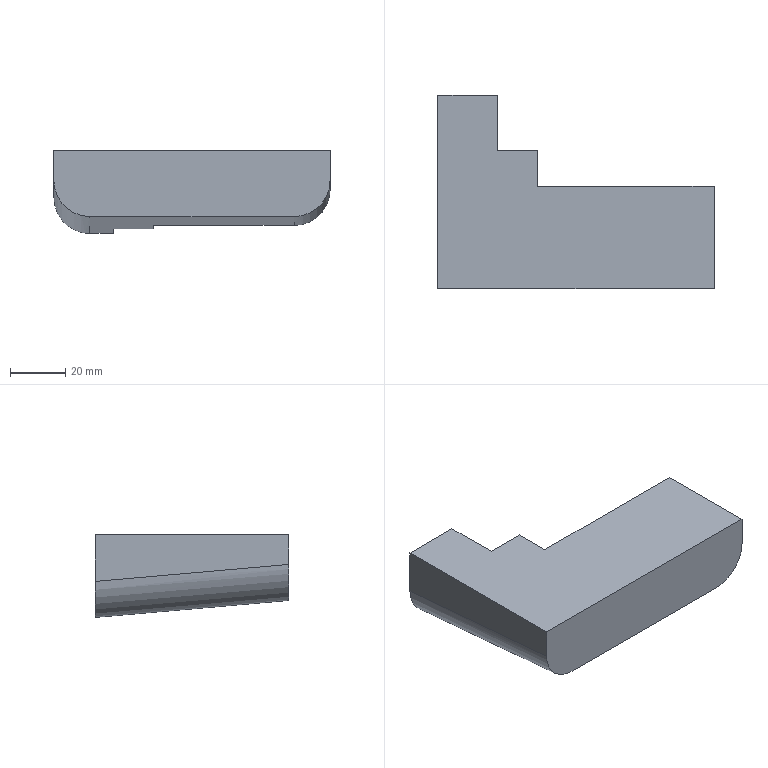Part | STEP file | 1 solid | 12 faces | box 100 x 70 x 30 mm | volume 115912 mm3 | plane 10 | cylinder 2 | commonest cylinder face diameters 26 x2
STEP:
#1=CARTESIAN_POINT('',(0.,0.,0.));
#2=DIRECTION('',(0.,0.,1.));
#3=DIRECTION('',(1.,0.,0.));
#4=AXIS2_PLACEMENT_3D('',#1,#2,#3);
#5=CARTESIAN_POINT('',(-86.362,50.,-64.721));
#6=VERTEX_POINT('',#5);
#7=CARTESIAN_POINT('',(-86.362,37.,-63.583));
#8=VERTEX_POINT('',#7);
#9=CARTESIAN_POINT('',(-86.362,70.,-66.47));
#10=DIRECTION('',(0.,-0.9962,0.08716));
#11=VECTOR('',#10,1.);
#12=LINE('',#9,#11);
#13=CARTESIAN_POINT('',(-72.362,70.,-66.47));
#14=DIRECTION('',(0.,0.08716,0.9962));
#15=DIRECTION('',(0.,-0.9962,0.08716));
#16=AXIS2_PLACEMENT_3D('',#13,#14,#15);
#17=PLANE('',#16);
#18=CARTESIAN_POINT('',(0.,-14.));
#19=DIRECTION('',(1.,0.));
#20=VECTOR('',#19,1.);
#21=LINE('',#18,#20);
#22=(GEOMETRIC_REPRESENTATION_CONTEXT(2)PARAMETRIC_REPRESENTATION_CONTEXT()REPRESENTATION_CONTEXT('',''));
#23=DEFINITIONAL_REPRESENTATION('',(#21),#22);
#24=PCURVE('',#17,#23);
#25=CARTESIAN_POINT('',(-86.362,0.,-92.47));
#26=DIRECTION('',(-1.,0.,0.));
#27=DIRECTION('',(0.,0.,1.));
#28=AXIS2_PLACEMENT_3D('',#25,#26,#27);
#29=PLANE('',#28);
#30=CARTESIAN_POINT('',(26.,70.));
#31=DIRECTION('',(0.08716,-0.9962));
#32=VECTOR('',#31,1.);
#33=LINE('',#30,#32);
#34=(GEOMETRIC_REPRESENTATION_CONTEXT(2)PARAMETRIC_REPRESENTATION_CONTEXT()REPRESENTATION_CONTEXT('',''));
#35=DEFINITIONAL_REPRESENTATION('',(#33),#34);
#36=PCURVE('',#29,#35);
#37=SURFACE_CURVE('',#12,(#24,#36),.PCURVE_S1.);
#38=EDGE_CURVE('',#6,#8,#37,.T.);
#39=ORIENTED_EDGE('',*,*,#38,.T.);
#40=CARTESIAN_POINT('',(-35.362,37.,-63.583));
#41=VERTEX_POINT('',#40);
#42=CARTESIAN_POINT('',(-72.362,37.,-63.583));
#43=DIRECTION('',(-1.,0.,0.));
#44=VECTOR('',#43,1.);
#45=LINE('',#42,#44);
#46=CARTESIAN_POINT('',(33.126,0.));
#47=DIRECTION('',(0.,-1.));
#48=VECTOR('',#47,1.);
#49=LINE('',#46,#48);
#50=(GEOMETRIC_REPRESENTATION_CONTEXT(2)PARAMETRIC_REPRESENTATION_CONTEXT()REPRESENTATION_CONTEXT('',''));
#51=DEFINITIONAL_REPRESENTATION('',(#49),#50);
#52=PCURVE('',#17,#51);
#53=CARTESIAN_POINT('',(-42.862,37.,-64.47));
#54=DIRECTION('',(0.,1.,0.));
#55=DIRECTION('',(0.,0.,1.));
#56=AXIS2_PLACEMENT_3D('',#53,#54,#55);
#57=PLANE('',#56);
#58=CARTESIAN_POINT('',(0.8871,-29.5));
#59=DIRECTION('',(0.,-1.));
#60=VECTOR('',#59,1.);
#61=LINE('',#58,#60);
#62=(GEOMETRIC_REPRESENTATION_CONTEXT(2)PARAMETRIC_REPRESENTATION_CONTEXT()REPRESENTATION_CONTEXT('',''));
#63=DEFINITIONAL_REPRESENTATION('',(#61),#62);
#64=PCURVE('',#57,#63);
#65=SURFACE_CURVE('',#45,(#52,#64),.PCURVE_S1.);
#66=EDGE_CURVE('',#41,#8,#65,.T.);
#67=ORIENTED_EDGE('',*,*,#66,.F.);
#68=CARTESIAN_POINT('',(-35.362,0.,-60.346));
#69=VERTEX_POINT('',#68);
#70=CARTESIAN_POINT('',(-35.362,70.,-66.47));
#71=DIRECTION('',(0.,0.9962,-0.08716));
#72=VECTOR('',#71,1.);
#73=LINE('',#70,#72);
#74=CARTESIAN_POINT('',(0.,37.));
#75=DIRECTION('',(-1.,0.));
#76=VECTOR('',#75,1.);
#77=LINE('',#74,#76);
#78=(GEOMETRIC_REPRESENTATION_CONTEXT(2)PARAMETRIC_REPRESENTATION_CONTEXT()REPRESENTATION_CONTEXT('',''));
#79=DEFINITIONAL_REPRESENTATION('',(#77),#78);
#80=PCURVE('',#17,#79);
#81=CARTESIAN_POINT('',(-35.362,149.657,-60.39));
#82=DIRECTION('',(0.,-0.9962,0.08716));
#83=DIRECTION('',(0.,-0.08716,-0.9962));
#84=AXIS2_PLACEMENT_3D('',#81,#82,#83);
#85=CYLINDRICAL_SURFACE('',#84,13.);
#86=CARTESIAN_POINT('',(0.,78.824));
#87=DIRECTION('',(0.,-1.));
#88=VECTOR('',#87,1.);
#89=LINE('',#86,#88);
#90=(GEOMETRIC_REPRESENTATION_CONTEXT(2)PARAMETRIC_REPRESENTATION_CONTEXT()REPRESENTATION_CONTEXT('',''));
#91=DEFINITIONAL_REPRESENTATION('',(#89),#90);
#92=PCURVE('',#85,#91);
#93=SURFACE_CURVE('',#73,(#80,#92),.PCURVE_S1.);
#94=EDGE_CURVE('',#69,#41,#93,.T.);
#95=ORIENTED_EDGE('',*,*,#94,.F.);
#96=CARTESIAN_POINT('',(-109.362,0.,-60.346));
#97=VERTEX_POINT('',#96);
#98=CARTESIAN_POINT('',(-72.362,0.,-60.346));
#99=DIRECTION('',(1.,0.,0.));
#100=VECTOR('',#99,1.);
#101=LINE('',#98,#100);
#102=CARTESIAN_POINT('',(70.267,0.));
#103=DIRECTION('',(0.,1.));
#104=VECTOR('',#103,1.);
#105=LINE('',#102,#104);
#106=(GEOMETRIC_REPRESENTATION_CONTEXT(2)PARAMETRIC_REPRESENTATION_CONTEXT()REPRESENTATION_CONTEXT('',''));
#107=DEFINITIONAL_REPRESENTATION('',(#105),#106);
#108=PCURVE('',#17,#107);
#109=CARTESIAN_POINT('',(-72.362,0.,-51.47));
#110=DIRECTION('',(0.,1.,0.));
#111=DIRECTION('',(-1.,0.,0.));
#112=AXIS2_PLACEMENT_3D('',#109,#110,#111);
#113=PLANE('',#112);
#114=CARTESIAN_POINT('',(0.,-8.876));
#115=DIRECTION('',(-1.,0.));
#116=VECTOR('',#115,1.);
#117=LINE('',#114,#116);
#118=(GEOMETRIC_REPRESENTATION_CONTEXT(2)PARAMETRIC_REPRESENTATION_CONTEXT()REPRESENTATION_CONTEXT('',''));
#119=DEFINITIONAL_REPRESENTATION('',(#117),#118);
#120=PCURVE('',#113,#119);
#121=SURFACE_CURVE('',#101,(#108,#120),.PCURVE_S1.);
#122=EDGE_CURVE('',#97,#69,#121,.T.);
#123=ORIENTED_EDGE('',*,*,#122,.F.);
#124=CARTESIAN_POINT('',(-109.362,70.,-66.47));
#125=VERTEX_POINT('',#124);
#126=CARTESIAN_POINT('',(-109.362,70.,-66.47));
#127=DIRECTION('',(0.,-0.9962,0.08716));
#128=VECTOR('',#127,1.);
#129=LINE('',#126,#128);
#130=CARTESIAN_POINT('',(0.,-37.));
#131=DIRECTION('',(1.,0.));
#132=VECTOR('',#131,1.);
#133=LINE('',#130,#132);
#134=(GEOMETRIC_REPRESENTATION_CONTEXT(2)PARAMETRIC_REPRESENTATION_CONTEXT()REPRESENTATION_CONTEXT('',''));
#135=DEFINITIONAL_REPRESENTATION('',(#133),#134);
#136=PCURVE('',#17,#135);
#137=CARTESIAN_POINT('',(-109.362,71.133,-53.52));
#138=DIRECTION('',(0.,-0.9962,0.08716));
#139=DIRECTION('',(0.,-0.08716,-0.9962));
#140=AXIS2_PLACEMENT_3D('',#137,#138,#139);
#141=CYLINDRICAL_SURFACE('',#140,13.);
#142=CARTESIAN_POINT('',(6.283,0.));
#143=DIRECTION('',(0.,1.));
#144=VECTOR('',#143,1.);
#145=LINE('',#142,#144);
#146=(GEOMETRIC_REPRESENTATION_CONTEXT(2)PARAMETRIC_REPRESENTATION_CONTEXT()REPRESENTATION_CONTEXT('',''));
#147=DEFINITIONAL_REPRESENTATION('',(#145),#146);
#148=PCURVE('',#141,#147);
#149=SURFACE_CURVE('',#129,(#136,#148),.PCURVE_S1.);
#150=EDGE_CURVE('',#125,#97,#149,.T.);
#151=ORIENTED_EDGE('',*,*,#150,.F.);
#152=CARTESIAN_POINT('',(-100.862,70.,-66.47));
#153=VERTEX_POINT('',#152);
#154=CARTESIAN_POINT('',(-72.362,70.,-66.47));
#155=DIRECTION('',(1.,0.,0.));
#156=VECTOR('',#155,1.);
#157=LINE('',#154,#156);
#158=CARTESIAN_POINT('',(0.,0.));
#159=DIRECTION('',(0.,1.));
#160=VECTOR('',#159,1.);
#161=LINE('',#158,#160);
#162=(GEOMETRIC_REPRESENTATION_CONTEXT(2)PARAMETRIC_REPRESENTATION_CONTEXT()REPRESENTATION_CONTEXT('',''));
#163=DEFINITIONAL_REPRESENTATION('',(#161),#162);
#164=PCURVE('',#17,#163);
#165=CARTESIAN_POINT('',(469.637,70.,73.53));
#166=DIRECTION('',(0.,-1.,0.));
#167=DIRECTION('',(1.,0.,0.));
#168=AXIS2_PLACEMENT_3D('',#165,#166,#167);
#169=PLANE('',#168);
#170=CARTESIAN_POINT('',(-542.,-140.));
#171=DIRECTION('',(1.,0.));
#172=VECTOR('',#171,1.);
#173=LINE('',#170,#172);
#174=(GEOMETRIC_REPRESENTATION_CONTEXT(2)PARAMETRIC_REPRESENTATION_CONTEXT()REPRESENTATION_CONTEXT('',''));
#175=DEFINITIONAL_REPRESENTATION('',(#173),#174);
#176=PCURVE('',#169,#175);
#177=SURFACE_CURVE('',#157,(#164,#176),.PCURVE_S1.);
#178=EDGE_CURVE('',#125,#153,#177,.T.);
#179=ORIENTED_EDGE('',*,*,#178,.T.);
#180=CARTESIAN_POINT('',(-100.862,50.,-64.721));
#181=VERTEX_POINT('',#180);
#182=CARTESIAN_POINT('',(-100.862,70.,-66.47));
#183=DIRECTION('',(0.,-0.9962,0.08716));
#184=VECTOR('',#183,1.);
#185=LINE('',#182,#184);
#186=CARTESIAN_POINT('',(0.,-28.5));
#187=DIRECTION('',(1.,0.));
#188=VECTOR('',#187,1.);
#189=LINE('',#186,#188);
#190=(GEOMETRIC_REPRESENTATION_CONTEXT(2)PARAMETRIC_REPRESENTATION_CONTEXT()REPRESENTATION_CONTEXT('',''));
#191=DEFINITIONAL_REPRESENTATION('',(#189),#190);
#192=PCURVE('',#17,#191);
#193=CARTESIAN_POINT('',(-100.862,0.,-92.47));
#194=DIRECTION('',(-1.,0.,0.));
#195=DIRECTION('',(0.,0.,1.));
#196=AXIS2_PLACEMENT_3D('',#193,#194,#195);
#197=PLANE('',#196);
#198=CARTESIAN_POINT('',(26.,70.));
#199=DIRECTION('',(0.08716,-0.9962));
#200=VECTOR('',#199,1.);
#201=LINE('',#198,#200);
#202=(GEOMETRIC_REPRESENTATION_CONTEXT(2)PARAMETRIC_REPRESENTATION_CONTEXT()REPRESENTATION_CONTEXT('',''));
#203=DEFINITIONAL_REPRESENTATION('',(#201),#202);
#204=PCURVE('',#197,#203);
#205=SURFACE_CURVE('',#185,(#192,#204),.PCURVE_S1.);
#206=EDGE_CURVE('',#153,#181,#205,.T.);
#207=ORIENTED_EDGE('',*,*,#206,.T.);
#208=CARTESIAN_POINT('',(-72.362,50.,-64.721));
#209=DIRECTION('',(-1.,0.,0.));
#210=VECTOR('',#209,1.);
#211=LINE('',#208,#210);
#212=CARTESIAN_POINT('',(20.076,0.));
#213=DIRECTION('',(0.,-1.));
#214=VECTOR('',#213,1.);
#215=LINE('',#212,#214);
#216=(GEOMETRIC_REPRESENTATION_CONTEXT(2)PARAMETRIC_REPRESENTATION_CONTEXT()REPRESENTATION_CONTEXT('',''));
#217=DEFINITIONAL_REPRESENTATION('',(#215),#216);
#218=PCURVE('',#17,#217);
#219=CARTESIAN_POINT('',(-100.862,50.,-92.47));
#220=DIRECTION('',(0.,1.,0.));
#221=DIRECTION('',(0.,0.,1.));
#222=AXIS2_PLACEMENT_3D('',#219,#220,#221);
#223=PLANE('',#222);
#224=CARTESIAN_POINT('',(27.75,28.5));
#225=DIRECTION('',(0.,-1.));
#226=VECTOR('',#225,1.);
#227=LINE('',#224,#226);
#228=(GEOMETRIC_REPRESENTATION_CONTEXT(2)PARAMETRIC_REPRESENTATION_CONTEXT()REPRESENTATION_CONTEXT('',''));
#229=DEFINITIONAL_REPRESENTATION('',(#227),#228);
#230=PCURVE('',#223,#229);
#231=SURFACE_CURVE('',#211,(#218,#230),.PCURVE_S1.);
#232=EDGE_CURVE('',#6,#181,#231,.T.);
#233=ORIENTED_EDGE('',*,*,#232,.F.);
#234=EDGE_LOOP('',(#39,#67,#95,#123,#151,#179,#207,#233));
#235=FACE_BOUND('',#234,.T.);
#236=ADVANCED_FACE('',(#235),#17,.F.);
#237=CARTESIAN_POINT('',(-22.363,37.,-36.47));
#238=VERTEX_POINT('',#237);
#239=CARTESIAN_POINT('',(-22.363,37.,-50.534));
#240=VERTEX_POINT('',#239);
#241=CARTESIAN_POINT('',(-22.363,37.,-56.47));
#242=DIRECTION('',(0.,0.,-1.));
#243=VECTOR('',#242,1.);
#244=LINE('',#241,#243);
#245=CARTESIAN_POINT('',(-22.363,150.,-56.47));
#246=DIRECTION('',(-1.,0.,0.));
#247=DIRECTION('',(0.,0.,-1.));
#248=AXIS2_PLACEMENT_3D('',#245,#246,#247);
#249=PLANE('',#248);
#250=CARTESIAN_POINT('',(0.,113.));
#251=DIRECTION('',(1.,0.));
#252=VECTOR('',#251,1.);
#253=LINE('',#250,#252);
#254=(GEOMETRIC_REPRESENTATION_CONTEXT(2)PARAMETRIC_REPRESENTATION_CONTEXT()REPRESENTATION_CONTEXT('',''));
#255=DEFINITIONAL_REPRESENTATION('',(#253),#254);
#256=PCURVE('',#249,#255);
#257=CARTESIAN_POINT('',(8.,20.5));
#258=DIRECTION('',(-1.,0.));
#259=VECTOR('',#258,1.);
#260=LINE('',#257,#259);
#261=(GEOMETRIC_REPRESENTATION_CONTEXT(2)PARAMETRIC_REPRESENTATION_CONTEXT()REPRESENTATION_CONTEXT('',''));
#262=DEFINITIONAL_REPRESENTATION('',(#260),#261);
#263=PCURVE('',#57,#262);
#264=SURFACE_CURVE('',#244,(#256,#263),.PCURVE_S1.);
#265=EDGE_CURVE('',#238,#240,#264,.T.);
#266=ORIENTED_EDGE('',*,*,#265,.F.);
#267=CARTESIAN_POINT('',(-22.363,0.,-36.47));
#268=VERTEX_POINT('',#267);
#269=CARTESIAN_POINT('',(-22.363,150.,-36.47));
#270=DIRECTION('',(0.,-1.,0.));
#271=VECTOR('',#270,1.);
#272=LINE('',#269,#271);
#273=CARTESIAN_POINT('',(-20.,0.));
#274=DIRECTION('',(0.,1.));
#275=VECTOR('',#274,1.);
#276=LINE('',#273,#275);
#277=(GEOMETRIC_REPRESENTATION_CONTEXT(2)PARAMETRIC_REPRESENTATION_CONTEXT()REPRESENTATION_CONTEXT('',''));
#278=DEFINITIONAL_REPRESENTATION('',(#276),#277);
#279=PCURVE('',#249,#278);
#280=CARTESIAN_POINT('',(-22.363,150.,-36.47));
#281=DIRECTION('',(0.,0.,-1.));
#282=DIRECTION('',(1.,0.,0.));
#283=AXIS2_PLACEMENT_3D('',#280,#281,#282);
#284=PLANE('',#283);
#285=CARTESIAN_POINT('',(0.,0.));
#286=DIRECTION('',(0.,1.));
#287=VECTOR('',#286,1.);
#288=LINE('',#285,#287);
#289=(GEOMETRIC_REPRESENTATION_CONTEXT(2)PARAMETRIC_REPRESENTATION_CONTEXT()REPRESENTATION_CONTEXT('',''));
#290=DEFINITIONAL_REPRESENTATION('',(#288),#289);
#291=PCURVE('',#284,#290);
#292=SURFACE_CURVE('',#272,(#279,#291),.PCURVE_S1.);
#293=EDGE_CURVE('',#238,#268,#292,.T.);
#294=ORIENTED_EDGE('',*,*,#293,.T.);
#295=CARTESIAN_POINT('',(-22.363,0.,-47.296));
#296=VERTEX_POINT('',#295);
#297=CARTESIAN_POINT('',(-22.363,0.,-56.47));
#298=DIRECTION('',(0.,0.,1.));
#299=VECTOR('',#298,1.);
#300=LINE('',#297,#299);
#301=CARTESIAN_POINT('',(0.,150.));
#302=DIRECTION('',(-1.,0.));
#303=VECTOR('',#302,1.);
#304=LINE('',#301,#303);
#305=(GEOMETRIC_REPRESENTATION_CONTEXT(2)PARAMETRIC_REPRESENTATION_CONTEXT()REPRESENTATION_CONTEXT('',''));
#306=DEFINITIONAL_REPRESENTATION('',(#304),#305);
#307=PCURVE('',#249,#306);
#308=CARTESIAN_POINT('',(-50.,-5.));
#309=DIRECTION('',(0.,1.));
#310=VECTOR('',#309,1.);
#311=LINE('',#308,#310);
#312=(GEOMETRIC_REPRESENTATION_CONTEXT(2)PARAMETRIC_REPRESENTATION_CONTEXT()REPRESENTATION_CONTEXT('',''));
#313=DEFINITIONAL_REPRESENTATION('',(#311),#312);
#314=PCURVE('',#113,#313);
#315=SURFACE_CURVE('',#300,(#307,#314),.PCURVE_S1.);
#316=EDGE_CURVE('',#296,#268,#315,.T.);
#317=ORIENTED_EDGE('',*,*,#316,.F.);
#318=CARTESIAN_POINT('',(-22.363,149.657,-60.39));
#319=DIRECTION('',(0.,-0.9962,0.08716));
#320=VECTOR('',#319,1.);
#321=LINE('',#318,#320);
#322=CARTESIAN_POINT('',(3.919,0.3429));
#323=DIRECTION('',(-0.08716,0.9962));
#324=VECTOR('',#323,1.);
#325=LINE('',#322,#324);
#326=(GEOMETRIC_REPRESENTATION_CONTEXT(2)PARAMETRIC_REPRESENTATION_CONTEXT()REPRESENTATION_CONTEXT('',''));
#327=DEFINITIONAL_REPRESENTATION('',(#325),#326);
#328=PCURVE('',#249,#327);
#329=CARTESIAN_POINT('',(1.571,0.));
#330=DIRECTION('',(0.,1.));
#331=VECTOR('',#330,1.);
#332=LINE('',#329,#331);
#333=(GEOMETRIC_REPRESENTATION_CONTEXT(2)PARAMETRIC_REPRESENTATION_CONTEXT()REPRESENTATION_CONTEXT('',''));
#334=DEFINITIONAL_REPRESENTATION('',(#332),#333);
#335=PCURVE('',#85,#334);
#336=SURFACE_CURVE('',#321,(#328,#335),.PCURVE_S1.);
#337=EDGE_CURVE('',#240,#296,#336,.T.);
#338=ORIENTED_EDGE('',*,*,#337,.F.);
#339=EDGE_LOOP('',(#266,#294,#317,#338));
#340=FACE_BOUND('',#339,.T.);
#341=ADVANCED_FACE('',(#340),#249,.F.);
#342=ORIENTED_EDGE('',*,*,#94,.T.);
#343=CARTESIAN_POINT('',(-35.362,37.,-63.583));
#344=CARTESIAN_POINT('',(-27.747,37.,-63.583));
#345=CARTESIAN_POINT('',(-22.363,37.,-58.178));
#346=CARTESIAN_POINT('',(-22.363,37.,-50.534));
#347=(BOUNDED_CURVE()B_SPLINE_CURVE(3,(#343,#344,#345,#346),.UNSPECIFIED.,.F.,.F.)B_SPLINE_CURVE_WITH_KNOTS((4,4),(3.142,4.712),.PIECEWISE_BEZIER_KNOTS.)CURVE()GEOMETRIC_REPRESENTATION_ITEM()RATIONAL_B_SPLINE_CURVE((1.,0.8047,0.8047,1.))REPRESENTATION_ITEM(''));
#348=CARTESIAN_POINT('',(0.,111.95));
#349=CARTESIAN_POINT('',(0.02143,111.95));
#350=CARTESIAN_POINT('',(0.06485,111.952));
#351=CARTESIAN_POINT('',(0.1316,111.959));
#352=CARTESIAN_POINT('',(0.2,111.972));
#353=CARTESIAN_POINT('',(0.2697,111.99));
#354=CARTESIAN_POINT('',(0.3408,112.015));
#355=CARTESIAN_POINT('',(0.413,112.045));
#356=CARTESIAN_POINT('',(0.4863,112.081));
#357=CARTESIAN_POINT('',(0.5603,112.123));
#358=CARTESIAN_POINT('',(0.635,112.171));
#359=CARTESIAN_POINT('',(0.7101,112.224));
#360=CARTESIAN_POINT('',(0.7854,112.282));
#361=CARTESIAN_POINT('',(0.8607,112.345));
#362=CARTESIAN_POINT('',(0.9358,112.412));
#363=CARTESIAN_POINT('',(1.01,112.482));
#364=CARTESIAN_POINT('',(1.085,112.555));
#365=CARTESIAN_POINT('',(1.158,112.631));
#366=CARTESIAN_POINT('',(1.23,112.707));
#367=CARTESIAN_POINT('',(1.301,112.784));
#368=CARTESIAN_POINT('',(1.371,112.861));
#369=CARTESIAN_POINT('',(1.439,112.938));
#370=CARTESIAN_POINT('',(1.506,113.014));
#371=CARTESIAN_POINT('',(1.549,113.063));
#372=CARTESIAN_POINT('',(1.571,113.087));
#373=B_SPLINE_CURVE_WITH_KNOTS('',3,(#348,#349,#350,#351,#352,#353,#354,#355,#356,#357,#358,#359,#360,#361,#362,#363,#364,#365,#366,#367,#368,#369,#370,#371,#372),.UNSPECIFIED.,.F.,.F.,(4,1,1,1,1,1,1,1,1,1,1,1,1,1,1,1,1,1,1,1,1,1,4),(3.142,3.213,3.284,3.356,3.427,3.499,3.57,3.641,3.713,3.784,3.856,3.927,3.998,4.07,4.141,4.213,4.284,4.355,4.427,4.498,4.57,4.641,4.712),.QUASI_UNIFORM_KNOTS.);
#374=(GEOMETRIC_REPRESENTATION_CONTEXT(2)PARAMETRIC_REPRESENTATION_CONTEXT()REPRESENTATION_CONTEXT('',''));
#375=DEFINITIONAL_REPRESENTATION('',(#373),#374);
#376=PCURVE('',#85,#375);
#377=CARTESIAN_POINT('',(0.8871,7.5));
#378=CARTESIAN_POINT('',(0.8871,15.115));
#379=CARTESIAN_POINT('',(6.292,20.5));
#380=CARTESIAN_POINT('',(13.937,20.5));
#381=(BOUNDED_CURVE()B_SPLINE_CURVE(3,(#377,#378,#379,#380),.UNSPECIFIED.,.F.,.F.)B_SPLINE_CURVE_WITH_KNOTS((4,4),(3.142,4.712),.PIECEWISE_BEZIER_KNOTS.)CURVE()GEOMETRIC_REPRESENTATION_ITEM()RATIONAL_B_SPLINE_CURVE((1.,0.8047,0.8047,1.))REPRESENTATION_ITEM(''));
#382=(GEOMETRIC_REPRESENTATION_CONTEXT(2)PARAMETRIC_REPRESENTATION_CONTEXT()REPRESENTATION_CONTEXT('',''));
#383=DEFINITIONAL_REPRESENTATION('',(#381),#382);
#384=PCURVE('',#57,#383);
#385=SURFACE_CURVE('',#347,(#376,#384),.PCURVE_S1.);
#386=EDGE_CURVE('',#41,#240,#385,.T.);
#387=ORIENTED_EDGE('',*,*,#386,.T.);
#388=ORIENTED_EDGE('',*,*,#337,.T.);
#389=CARTESIAN_POINT('',(-22.363,0.,-47.296));
#390=CARTESIAN_POINT('',(-22.363,0.,-54.941));
#391=CARTESIAN_POINT('',(-27.747,0.,-60.346));
#392=CARTESIAN_POINT('',(-35.362,0.,-60.346));
#393=(BOUNDED_CURVE()B_SPLINE_CURVE(3,(#389,#390,#391,#392),.UNSPECIFIED.,.F.,.F.)B_SPLINE_CURVE_WITH_KNOTS((4,4),(1.571,3.142),.PIECEWISE_BEZIER_KNOTS.)CURVE()GEOMETRIC_REPRESENTATION_ITEM()RATIONAL_B_SPLINE_CURVE((1.,0.8047,0.8047,1.))REPRESENTATION_ITEM(''));
#394=CARTESIAN_POINT('',(1.571,150.229));
#395=CARTESIAN_POINT('',(1.549,150.204));
#396=CARTESIAN_POINT('',(1.506,150.155));
#397=CARTESIAN_POINT('',(1.439,150.079));
#398=CARTESIAN_POINT('',(1.371,150.003));
#399=CARTESIAN_POINT('',(1.301,149.925));
#400=CARTESIAN_POINT('',(1.23,149.848));
#401=CARTESIAN_POINT('',(1.158,149.772));
#402=CARTESIAN_POINT('',(1.085,149.697));
#403=CARTESIAN_POINT('',(1.01,149.624));
#404=CARTESIAN_POINT('',(0.9358,149.553));
#405=CARTESIAN_POINT('',(0.8607,149.487));
#406=CARTESIAN_POINT('',(0.7854,149.424));
#407=CARTESIAN_POINT('',(0.7101,149.365));
#408=CARTESIAN_POINT('',(0.635,149.312));
#409=CARTESIAN_POINT('',(0.5603,149.264));
#410=CARTESIAN_POINT('',(0.4863,149.222));
#411=CARTESIAN_POINT('',(0.413,149.186));
#412=CARTESIAN_POINT('',(0.3408,149.156));
#413=CARTESIAN_POINT('',(0.2697,149.132));
#414=CARTESIAN_POINT('',(0.2,149.113));
#415=CARTESIAN_POINT('',(0.1316,149.1));
#416=CARTESIAN_POINT('',(0.06485,149.093));
#417=CARTESIAN_POINT('',(0.02143,149.091));
#418=CARTESIAN_POINT('',(0.,149.091));
#419=B_SPLINE_CURVE_WITH_KNOTS('',3,(#394,#395,#396,#397,#398,#399,#400,#401,#402,#403,#404,#405,#406,#407,#408,#409,#410,#411,#412,#413,#414,#415,#416,#417,#418),.UNSPECIFIED.,.F.,.F.,(4,1,1,1,1,1,1,1,1,1,1,1,1,1,1,1,1,1,1,1,1,1,4),(1.571,1.642,1.714,1.785,1.856,1.928,1.999,2.071,2.142,2.213,2.285,2.356,2.428,2.499,2.57,2.642,2.713,2.785,2.856,2.927,2.999,3.07,3.142),.QUASI_UNIFORM_KNOTS.);
#420=(GEOMETRIC_REPRESENTATION_CONTEXT(2)PARAMETRIC_REPRESENTATION_CONTEXT()REPRESENTATION_CONTEXT('',''));
#421=DEFINITIONAL_REPRESENTATION('',(#419),#420);
#422=PCURVE('',#85,#421);
#423=CARTESIAN_POINT('',(-50.,4.174));
#424=CARTESIAN_POINT('',(-50.,-3.47));
#425=CARTESIAN_POINT('',(-44.615,-8.876));
#426=CARTESIAN_POINT('',(-37.,-8.876));
#427=(BOUNDED_CURVE()B_SPLINE_CURVE(3,(#423,#424,#425,#426),.UNSPECIFIED.,.F.,.F.)B_SPLINE_CURVE_WITH_KNOTS((4,4),(1.571,3.142),.PIECEWISE_BEZIER_KNOTS.)CURVE()GEOMETRIC_REPRESENTATION_ITEM()RATIONAL_B_SPLINE_CURVE((1.,0.8047,0.8047,1.))REPRESENTATION_ITEM(''));
#428=(GEOMETRIC_REPRESENTATION_CONTEXT(2)PARAMETRIC_REPRESENTATION_CONTEXT()REPRESENTATION_CONTEXT('',''));
#429=DEFINITIONAL_REPRESENTATION('',(#427),#428);
#430=PCURVE('',#113,#429);
#431=SURFACE_CURVE('',#393,(#422,#430),.PCURVE_S1.);
#432=EDGE_CURVE('',#296,#69,#431,.T.);
#433=ORIENTED_EDGE('',*,*,#432,.T.);
#434=EDGE_LOOP('',(#342,#387,#388,#433));
#435=FACE_BOUND('',#434,.T.);
#436=ADVANCED_FACE('',(#435),#85,.T.);
#437=CARTESIAN_POINT('',(-86.362,37.,-36.47));
#438=VERTEX_POINT('',#437);
#439=CARTESIAN_POINT('',(-22.363,37.,-36.47));
#440=DIRECTION('',(-1.,0.,0.));
#441=VECTOR('',#440,1.);
#442=LINE('',#439,#441);
#443=CARTESIAN_POINT('',(0.,113.));
#444=DIRECTION('',(-1.,0.));
#445=VECTOR('',#444,1.);
#446=LINE('',#443,#445);
#447=(GEOMETRIC_REPRESENTATION_CONTEXT(2)PARAMETRIC_REPRESENTATION_CONTEXT()REPRESENTATION_CONTEXT('',''));
#448=DEFINITIONAL_REPRESENTATION('',(#446),#447);
#449=PCURVE('',#284,#448);
#450=CARTESIAN_POINT('',(28.,20.5));
#451=DIRECTION('',(0.,-1.));
#452=VECTOR('',#451,1.);
#453=LINE('',#450,#452);
#454=(GEOMETRIC_REPRESENTATION_CONTEXT(2)PARAMETRIC_REPRESENTATION_CONTEXT()REPRESENTATION_CONTEXT('',''));
#455=DEFINITIONAL_REPRESENTATION('',(#453),#454);
#456=PCURVE('',#57,#455);
#457=SURFACE_CURVE('',#442,(#449,#456),.PCURVE_S1.);
#458=EDGE_CURVE('',#238,#438,#457,.T.);
#459=ORIENTED_EDGE('',*,*,#458,.T.);
#460=CARTESIAN_POINT('',(-86.362,50.,-36.47));
#461=VERTEX_POINT('',#460);
#462=CARTESIAN_POINT('',(-86.362,150.,-36.47));
#463=DIRECTION('',(0.,1.,0.));
#464=VECTOR('',#463,1.);
#465=LINE('',#462,#464);
#466=CARTESIAN_POINT('',(-64.,0.));
#467=DIRECTION('',(0.,-1.));
#468=VECTOR('',#467,1.);
#469=LINE('',#466,#468);
#470=(GEOMETRIC_REPRESENTATION_CONTEXT(2)PARAMETRIC_REPRESENTATION_CONTEXT()REPRESENTATION_CONTEXT('',''));
#471=DEFINITIONAL_REPRESENTATION('',(#469),#470);
#472=PCURVE('',#284,#471);
#473=CARTESIAN_POINT('',(56.,150.));
#474=DIRECTION('',(0.,1.));
#475=VECTOR('',#474,1.);
#476=LINE('',#473,#475);
#477=(GEOMETRIC_REPRESENTATION_CONTEXT(2)PARAMETRIC_REPRESENTATION_CONTEXT()REPRESENTATION_CONTEXT('',''));
#478=DEFINITIONAL_REPRESENTATION('',(#476),#477);
#479=PCURVE('',#29,#478);
#480=SURFACE_CURVE('',#465,(#472,#479),.PCURVE_S1.);
#481=EDGE_CURVE('',#438,#461,#480,.T.);
#482=ORIENTED_EDGE('',*,*,#481,.T.);
#483=CARTESIAN_POINT('',(-100.862,50.,-36.47));
#484=VERTEX_POINT('',#483);
#485=CARTESIAN_POINT('',(-100.862,50.,-36.47));
#486=DIRECTION('',(1.,0.,0.));
#487=VECTOR('',#486,1.);
#488=LINE('',#485,#487);
#489=CARTESIAN_POINT('',(-78.5,100.));
#490=DIRECTION('',(1.,0.));
#491=VECTOR('',#490,1.);
#492=LINE('',#489,#491);
#493=(GEOMETRIC_REPRESENTATION_CONTEXT(2)PARAMETRIC_REPRESENTATION_CONTEXT()REPRESENTATION_CONTEXT('',''));
#494=DEFINITIONAL_REPRESENTATION('',(#492),#493);
#495=PCURVE('',#284,#494);
#496=CARTESIAN_POINT('',(56.,0.));
#497=DIRECTION('',(0.,1.));
#498=VECTOR('',#497,1.);
#499=LINE('',#496,#498);
#500=(GEOMETRIC_REPRESENTATION_CONTEXT(2)PARAMETRIC_REPRESENTATION_CONTEXT()REPRESENTATION_CONTEXT('',''));
#501=DEFINITIONAL_REPRESENTATION('',(#499),#500);
#502=PCURVE('',#223,#501);
#503=SURFACE_CURVE('',#488,(#495,#502),.PCURVE_S1.);
#504=EDGE_CURVE('',#484,#461,#503,.T.);
#505=ORIENTED_EDGE('',*,*,#504,.F.);
#506=CARTESIAN_POINT('',(-100.862,70.,-36.47));
#507=VERTEX_POINT('',#506);
#508=CARTESIAN_POINT('',(-100.862,90.366,-36.47));
#509=DIRECTION('',(0.,-1.,0.));
#510=VECTOR('',#509,1.);
#511=LINE('',#508,#510);
#512=CARTESIAN_POINT('',(-78.5,59.634));
#513=DIRECTION('',(0.,1.));
#514=VECTOR('',#513,1.);
#515=LINE('',#512,#514);
#516=(GEOMETRIC_REPRESENTATION_CONTEXT(2)PARAMETRIC_REPRESENTATION_CONTEXT()REPRESENTATION_CONTEXT('',''));
#517=DEFINITIONAL_REPRESENTATION('',(#515),#516);
#518=PCURVE('',#284,#517);
#519=CARTESIAN_POINT('',(56.,90.366));
#520=DIRECTION('',(0.,-1.));
#521=VECTOR('',#520,1.);
#522=LINE('',#519,#521);
#523=(GEOMETRIC_REPRESENTATION_CONTEXT(2)PARAMETRIC_REPRESENTATION_CONTEXT()REPRESENTATION_CONTEXT('',''));
#524=DEFINITIONAL_REPRESENTATION('',(#522),#523);
#525=PCURVE('',#197,#524);
#526=SURFACE_CURVE('',#511,(#518,#525),.PCURVE_S1.);
#527=EDGE_CURVE('',#507,#484,#526,.T.);
#528=ORIENTED_EDGE('',*,*,#527,.F.);
#529=CARTESIAN_POINT('',(-122.362,70.,-36.47));
#530=VERTEX_POINT('',#529);
#531=CARTESIAN_POINT('',(-22.363,70.,-36.47));
#532=DIRECTION('',(-1.,0.,0.));
#533=VECTOR('',#532,1.);
#534=LINE('',#531,#533);
#535=CARTESIAN_POINT('',(0.,80.));
#536=DIRECTION('',(-1.,0.));
#537=VECTOR('',#536,1.);
#538=LINE('',#535,#537);
#539=(GEOMETRIC_REPRESENTATION_CONTEXT(2)PARAMETRIC_REPRESENTATION_CONTEXT()REPRESENTATION_CONTEXT('',''));
#540=DEFINITIONAL_REPRESENTATION('',(#538),#539);
#541=PCURVE('',#284,#540);
#542=CARTESIAN_POINT('',(-492.,-110.));
#543=DIRECTION('',(-1.,0.));
#544=VECTOR('',#543,1.);
#545=LINE('',#542,#544);
#546=(GEOMETRIC_REPRESENTATION_CONTEXT(2)PARAMETRIC_REPRESENTATION_CONTEXT()REPRESENTATION_CONTEXT('',''));
#547=DEFINITIONAL_REPRESENTATION('',(#545),#546);
#548=PCURVE('',#169,#547);
#549=SURFACE_CURVE('',#534,(#541,#548),.PCURVE_S1.);
#550=EDGE_CURVE('',#507,#530,#549,.T.);
#551=ORIENTED_EDGE('',*,*,#550,.T.);
#552=CARTESIAN_POINT('',(-122.362,0.,-36.47));
#553=VERTEX_POINT('',#552);
#554=CARTESIAN_POINT('',(-122.362,150.,-36.47));
#555=DIRECTION('',(0.,-1.,0.));
#556=VECTOR('',#555,1.);
#557=LINE('',#554,#556);
#558=CARTESIAN_POINT('',(-100.,0.));
#559=DIRECTION('',(0.,1.));
#560=VECTOR('',#559,1.);
#561=LINE('',#558,#560);
#562=(GEOMETRIC_REPRESENTATION_CONTEXT(2)PARAMETRIC_REPRESENTATION_CONTEXT()REPRESENTATION_CONTEXT('',''));
#563=DEFINITIONAL_REPRESENTATION('',(#561),#562);
#564=PCURVE('',#284,#563);
#565=CARTESIAN_POINT('',(-122.362,150.,-36.47));
#566=DIRECTION('',(1.,0.,0.));
#567=DIRECTION('',(0.,0.,1.));
#568=AXIS2_PLACEMENT_3D('',#565,#566,#567);
#569=PLANE('',#568);
#570=CARTESIAN_POINT('',(0.,0.));
#571=DIRECTION('',(0.,1.));
#572=VECTOR('',#571,1.);
#573=LINE('',#570,#572);
#574=(GEOMETRIC_REPRESENTATION_CONTEXT(2)PARAMETRIC_REPRESENTATION_CONTEXT()REPRESENTATION_CONTEXT('',''));
#575=DEFINITIONAL_REPRESENTATION('',(#573),#574);
#576=PCURVE('',#569,#575);
#577=SURFACE_CURVE('',#557,(#564,#576),.PCURVE_S1.);
#578=EDGE_CURVE('',#530,#553,#577,.T.);
#579=ORIENTED_EDGE('',*,*,#578,.T.);
#580=CARTESIAN_POINT('',(-22.363,0.,-36.47));
#581=DIRECTION('',(-1.,0.,0.));
#582=VECTOR('',#581,1.);
#583=LINE('',#580,#582);
#584=CARTESIAN_POINT('',(0.,150.));
#585=DIRECTION('',(-1.,0.));
#586=VECTOR('',#585,1.);
#587=LINE('',#584,#586);
#588=(GEOMETRIC_REPRESENTATION_CONTEXT(2)PARAMETRIC_REPRESENTATION_CONTEXT()REPRESENTATION_CONTEXT('',''));
#589=DEFINITIONAL_REPRESENTATION('',(#587),#588);
#590=PCURVE('',#284,#589);
#591=CARTESIAN_POINT('',(-50.,15.));
#592=DIRECTION('',(1.,0.));
#593=VECTOR('',#592,1.);
#594=LINE('',#591,#593);
#595=(GEOMETRIC_REPRESENTATION_CONTEXT(2)PARAMETRIC_REPRESENTATION_CONTEXT()REPRESENTATION_CONTEXT('',''));
#596=DEFINITIONAL_REPRESENTATION('',(#594),#595);
#597=PCURVE('',#113,#596);
#598=SURFACE_CURVE('',#583,(#590,#597),.PCURVE_S1.);
#599=EDGE_CURVE('',#268,#553,#598,.T.);
#600=ORIENTED_EDGE('',*,*,#599,.F.);
#601=ORIENTED_EDGE('',*,*,#293,.F.);
#602=EDGE_LOOP('',(#459,#482,#505,#528,#551,#579,#600,#601));
#603=FACE_BOUND('',#602,.T.);
#604=ADVANCED_FACE('',(#603),#284,.F.);
#605=CARTESIAN_POINT('',(-100.862,70.,-363.47));
#606=DIRECTION('',(0.,0.,1.));
#607=VECTOR('',#606,1.);
#608=LINE('',#605,#607);
#609=CARTESIAN_POINT('',(-570.5,-437.));
#610=DIRECTION('',(0.,1.));
#611=VECTOR('',#610,1.);
#612=LINE('',#609,#611);
#613=(GEOMETRIC_REPRESENTATION_CONTEXT(2)PARAMETRIC_REPRESENTATION_CONTEXT()REPRESENTATION_CONTEXT('',''));
#614=DEFINITIONAL_REPRESENTATION('',(#612),#613);
#615=PCURVE('',#169,#614);
#616=CARTESIAN_POINT('',(-271.,70.));
#617=DIRECTION('',(1.,0.));
#618=VECTOR('',#617,1.);
#619=LINE('',#616,#618);
#620=(GEOMETRIC_REPRESENTATION_CONTEXT(2)PARAMETRIC_REPRESENTATION_CONTEXT()REPRESENTATION_CONTEXT('',''));
#621=DEFINITIONAL_REPRESENTATION('',(#619),#620);
#622=PCURVE('',#197,#621);
#623=SURFACE_CURVE('',#608,(#615,#622),.PCURVE_S1.);
#624=EDGE_CURVE('',#153,#507,#623,.T.);
#625=ORIENTED_EDGE('',*,*,#624,.F.);
#626=ORIENTED_EDGE('',*,*,#178,.F.);
#627=CARTESIAN_POINT('',(-122.362,70.,-53.421));
#628=VERTEX_POINT('',#627);
#629=CARTESIAN_POINT('',(-122.362,70.,-53.421));
#630=CARTESIAN_POINT('',(-122.362,70.,-61.065));
#631=CARTESIAN_POINT('',(-116.978,70.,-66.47));
#632=CARTESIAN_POINT('',(-109.362,70.,-66.47));
#633=(BOUNDED_CURVE()B_SPLINE_CURVE(3,(#629,#630,#631,#632),.UNSPECIFIED.,.F.,.F.)B_SPLINE_CURVE_WITH_KNOTS((4,4),(1.571,3.142),.PIECEWISE_BEZIER_KNOTS.)CURVE()GEOMETRIC_REPRESENTATION_ITEM()RATIONAL_B_SPLINE_CURVE((1.,0.8047,0.8047,1.))REPRESENTATION_ITEM(''));
#634=CARTESIAN_POINT('',(-592.,-126.95));
#635=CARTESIAN_POINT('',(-592.,-134.595));
#636=CARTESIAN_POINT('',(-586.615,-140.));
#637=CARTESIAN_POINT('',(-579.,-140.));
#638=(BOUNDED_CURVE()B_SPLINE_CURVE(3,(#634,#635,#636,#637),.UNSPECIFIED.,.F.,.F.)B_SPLINE_CURVE_WITH_KNOTS((4,4),(1.571,3.142),.PIECEWISE_BEZIER_KNOTS.)CURVE()GEOMETRIC_REPRESENTATION_ITEM()RATIONAL_B_SPLINE_CURVE((1.,0.8047,0.8047,1.))REPRESENTATION_ITEM(''));
#639=(GEOMETRIC_REPRESENTATION_CONTEXT(2)PARAMETRIC_REPRESENTATION_CONTEXT()REPRESENTATION_CONTEXT('',''));
#640=DEFINITIONAL_REPRESENTATION('',(#638),#639);
#641=PCURVE('',#169,#640);
#642=CARTESIAN_POINT('',(4.712,1.137));
#643=CARTESIAN_POINT('',(4.734,1.113));
#644=CARTESIAN_POINT('',(4.777,1.064));
#645=CARTESIAN_POINT('',(4.844,0.988));
#646=CARTESIAN_POINT('',(4.912,0.9113));
#647=CARTESIAN_POINT('',(4.982,0.834));
#648=CARTESIAN_POINT('',(5.053,0.7569));
#649=CARTESIAN_POINT('',(5.125,0.6804));
#650=CARTESIAN_POINT('',(5.199,0.6054));
#651=CARTESIAN_POINT('',(5.273,0.5323));
#652=CARTESIAN_POINT('',(5.347,0.4621));
#653=CARTESIAN_POINT('',(5.422,0.3952));
#654=CARTESIAN_POINT('',(5.498,0.3324));
#655=CARTESIAN_POINT('',(5.573,0.2741));
#656=CARTESIAN_POINT('',(5.648,0.2208));
#657=CARTESIAN_POINT('',(5.723,0.173));
#658=CARTESIAN_POINT('',(5.797,0.1309));
#659=CARTESIAN_POINT('',(5.87,0.09472));
#660=CARTESIAN_POINT('',(5.942,0.06449));
#661=CARTESIAN_POINT('',(6.013,0.04021));
#662=CARTESIAN_POINT('',(6.083,0.02178));
#663=CARTESIAN_POINT('',(6.152,0.008981));
#664=CARTESIAN_POINT('',(6.218,0.001569));
#665=CARTESIAN_POINT('',(6.262,-0.000003694));
#666=CARTESIAN_POINT('',(6.283,0.));
#667=B_SPLINE_CURVE_WITH_KNOTS('',3,(#642,#643,#644,#645,#646,#647,#648,#649,#650,#651,#652,#653,#654,#655,#656,#657,#658,#659,#660,#661,#662,#663,#664,#665,#666),.UNSPECIFIED.,.F.,.F.,(4,1,1,1,1,1,1,1,1,1,1,1,1,1,1,1,1,1,1,1,1,1,4),(1.571,1.642,1.714,1.785,1.856,1.928,1.999,2.071,2.142,2.213,2.285,2.356,2.428,2.499,2.57,2.642,2.713,2.785,2.856,2.927,2.999,3.07,3.142),.QUASI_UNIFORM_KNOTS.);
#668=(GEOMETRIC_REPRESENTATION_CONTEXT(2)PARAMETRIC_REPRESENTATION_CONTEXT()REPRESENTATION_CONTEXT('',''));
#669=DEFINITIONAL_REPRESENTATION('',(#667),#668);
#670=PCURVE('',#141,#669);
#671=SURFACE_CURVE('',#633,(#641,#670),.PCURVE_S1.);
#672=EDGE_CURVE('',#628,#125,#671,.T.);
#673=ORIENTED_EDGE('',*,*,#672,.F.);
#674=CARTESIAN_POINT('',(-122.362,70.,-36.47));
#675=DIRECTION('',(0.,0.,-1.));
#676=VECTOR('',#675,1.);
#677=LINE('',#674,#676);
#678=CARTESIAN_POINT('',(-592.,-110.));
#679=DIRECTION('',(0.,-1.));
#680=VECTOR('',#679,1.);
#681=LINE('',#678,#680);
#682=(GEOMETRIC_REPRESENTATION_CONTEXT(2)PARAMETRIC_REPRESENTATION_CONTEXT()REPRESENTATION_CONTEXT('',''));
#683=DEFINITIONAL_REPRESENTATION('',(#681),#682);
#684=PCURVE('',#169,#683);
#685=CARTESIAN_POINT('',(0.,80.));
#686=DIRECTION('',(-1.,0.));
#687=VECTOR('',#686,1.);
#688=LINE('',#685,#687);
#689=(GEOMETRIC_REPRESENTATION_CONTEXT(2)PARAMETRIC_REPRESENTATION_CONTEXT()REPRESENTATION_CONTEXT('',''));
#690=DEFINITIONAL_REPRESENTATION('',(#688),#689);
#691=PCURVE('',#569,#690);
#692=SURFACE_CURVE('',#677,(#684,#691),.PCURVE_S1.);
#693=EDGE_CURVE('',#530,#628,#692,.T.);
#694=ORIENTED_EDGE('',*,*,#693,.F.);
#695=ORIENTED_EDGE('',*,*,#550,.F.);
#696=EDGE_LOOP('',(#625,#626,#673,#694,#695));
#697=FACE_BOUND('',#696,.T.);
#698=ADVANCED_FACE('',(#697),#169,.F.);
#699=CARTESIAN_POINT('',(-122.362,0.,-47.296));
#700=VERTEX_POINT('',#699);
#701=CARTESIAN_POINT('',(-122.362,0.,-36.47));
#702=DIRECTION('',(0.,0.,-1.));
#703=VECTOR('',#702,1.);
#704=LINE('',#701,#703);
#705=CARTESIAN_POINT('',(0.,150.));
#706=DIRECTION('',(-1.,0.));
#707=VECTOR('',#706,1.);
#708=LINE('',#705,#707);
#709=(GEOMETRIC_REPRESENTATION_CONTEXT(2)PARAMETRIC_REPRESENTATION_CONTEXT()REPRESENTATION_CONTEXT('',''));
#710=DEFINITIONAL_REPRESENTATION('',(#708),#709);
#711=PCURVE('',#569,#710);
#712=CARTESIAN_POINT('',(50.,15.));
#713=DIRECTION('',(0.,-1.));
#714=VECTOR('',#713,1.);
#715=LINE('',#712,#714);
#716=(GEOMETRIC_REPRESENTATION_CONTEXT(2)PARAMETRIC_REPRESENTATION_CONTEXT()REPRESENTATION_CONTEXT('',''));
#717=DEFINITIONAL_REPRESENTATION('',(#715),#716);
#718=PCURVE('',#113,#717);
#719=SURFACE_CURVE('',#704,(#711,#718),.PCURVE_S1.);
#720=EDGE_CURVE('',#553,#700,#719,.T.);
#721=ORIENTED_EDGE('',*,*,#720,.F.);
#722=ORIENTED_EDGE('',*,*,#578,.F.);
#723=ORIENTED_EDGE('',*,*,#693,.T.);
#724=CARTESIAN_POINT('',(-122.362,147.921,-60.238));
#725=DIRECTION('',(0.,0.9962,-0.08716));
#726=VECTOR('',#725,1.);
#727=LINE('',#724,#726);
#728=CARTESIAN_POINT('',(-23.768,2.079));
#729=DIRECTION('',(-0.08716,-0.9962));
#730=VECTOR('',#729,1.);
#731=LINE('',#728,#730);
#732=(GEOMETRIC_REPRESENTATION_CONTEXT(2)PARAMETRIC_REPRESENTATION_CONTEXT()REPRESENTATION_CONTEXT('',''));
#733=DEFINITIONAL_REPRESENTATION('',(#731),#732);
#734=PCURVE('',#569,#733);
#735=CARTESIAN_POINT('',(4.712,-77.081));
#736=DIRECTION('',(0.,-1.));
#737=VECTOR('',#736,1.);
#738=LINE('',#735,#737);
#739=(GEOMETRIC_REPRESENTATION_CONTEXT(2)PARAMETRIC_REPRESENTATION_CONTEXT()REPRESENTATION_CONTEXT('',''));
#740=DEFINITIONAL_REPRESENTATION('',(#738),#739);
#741=PCURVE('',#141,#740);
#742=SURFACE_CURVE('',#727,(#734,#741),.PCURVE_S1.);
#743=EDGE_CURVE('',#700,#628,#742,.T.);
#744=ORIENTED_EDGE('',*,*,#743,.F.);
#745=EDGE_LOOP('',(#721,#722,#723,#744));
#746=FACE_BOUND('',#745,.T.);
#747=ADVANCED_FACE('',(#746),#569,.F.);
#748=ORIENTED_EDGE('',*,*,#122,.T.);
#749=ORIENTED_EDGE('',*,*,#432,.F.);
#750=ORIENTED_EDGE('',*,*,#316,.T.);
#751=ORIENTED_EDGE('',*,*,#599,.T.);
#752=ORIENTED_EDGE('',*,*,#720,.T.);
#753=CARTESIAN_POINT('',(-109.362,0.,-60.346));
#754=CARTESIAN_POINT('',(-116.978,0.,-60.346));
#755=CARTESIAN_POINT('',(-122.362,0.,-54.941));
#756=CARTESIAN_POINT('',(-122.362,0.,-47.296));
#757=(BOUNDED_CURVE()B_SPLINE_CURVE(3,(#753,#754,#755,#756),.UNSPECIFIED.,.F.,.F.)B_SPLINE_CURVE_WITH_KNOTS((4,4),(3.142,4.712),.PIECEWISE_BEZIER_KNOTS.)CURVE()GEOMETRIC_REPRESENTATION_ITEM()RATIONAL_B_SPLINE_CURVE((1.,0.8047,0.8047,1.))REPRESENTATION_ITEM(''));
#758=CARTESIAN_POINT('',(37.,-8.876));
#759=CARTESIAN_POINT('',(44.615,-8.876));
#760=CARTESIAN_POINT('',(50.,-3.47));
#761=CARTESIAN_POINT('',(50.,4.174));
#762=(BOUNDED_CURVE()B_SPLINE_CURVE(3,(#758,#759,#760,#761),.UNSPECIFIED.,.F.,.F.)B_SPLINE_CURVE_WITH_KNOTS((4,4),(3.142,4.712),.PIECEWISE_BEZIER_KNOTS.)CURVE()GEOMETRIC_REPRESENTATION_ITEM()RATIONAL_B_SPLINE_CURVE((1.,0.8047,0.8047,1.))REPRESENTATION_ITEM(''));
#763=(GEOMETRIC_REPRESENTATION_CONTEXT(2)PARAMETRIC_REPRESENTATION_CONTEXT()REPRESENTATION_CONTEXT('',''));
#764=DEFINITIONAL_REPRESENTATION('',(#762),#763);
#765=PCURVE('',#113,#764);
#766=CARTESIAN_POINT('',(6.283,70.267));
#767=CARTESIAN_POINT('',(6.262,70.267));
#768=CARTESIAN_POINT('',(6.218,70.269));
#769=CARTESIAN_POINT('',(6.152,70.276));
#770=CARTESIAN_POINT('',(6.083,70.289));
#771=CARTESIAN_POINT('',(6.013,70.308));
#772=CARTESIAN_POINT('',(5.942,70.332));
#773=CARTESIAN_POINT('',(5.87,70.362));
#774=CARTESIAN_POINT('',(5.797,70.398));
#775=CARTESIAN_POINT('',(5.723,70.44));
#776=CARTESIAN_POINT('',(5.648,70.488));
#777=CARTESIAN_POINT('',(5.573,70.541));
#778=CARTESIAN_POINT('',(5.498,70.6));
#779=CARTESIAN_POINT('',(5.422,70.663));
#780=CARTESIAN_POINT('',(5.347,70.729));
#781=CARTESIAN_POINT('',(5.273,70.8));
#782=CARTESIAN_POINT('',(5.199,70.873));
#783=CARTESIAN_POINT('',(5.125,70.948));
#784=CARTESIAN_POINT('',(5.053,71.024));
#785=CARTESIAN_POINT('',(4.982,71.101));
#786=CARTESIAN_POINT('',(4.912,71.179));
#787=CARTESIAN_POINT('',(4.844,71.255));
#788=CARTESIAN_POINT('',(4.777,71.331));
#789=CARTESIAN_POINT('',(4.734,71.38));
#790=CARTESIAN_POINT('',(4.712,71.405));
#791=B_SPLINE_CURVE_WITH_KNOTS('',3,(#766,#767,#768,#769,#770,#771,#772,#773,#774,#775,#776,#777,#778,#779,#780,#781,#782,#783,#784,#785,#786,#787,#788,#789,#790),.UNSPECIFIED.,.F.,.F.,(4,1,1,1,1,1,1,1,1,1,1,1,1,1,1,1,1,1,1,1,1,1,4),(3.142,3.213,3.284,3.356,3.427,3.499,3.57,3.641,3.713,3.784,3.856,3.927,3.998,4.07,4.141,4.213,4.284,4.355,4.427,4.498,4.57,4.641,4.712),.QUASI_UNIFORM_KNOTS.);
#792=(GEOMETRIC_REPRESENTATION_CONTEXT(2)PARAMETRIC_REPRESENTATION_CONTEXT()REPRESENTATION_CONTEXT('',''));
#793=DEFINITIONAL_REPRESENTATION('',(#791),#792);
#794=PCURVE('',#141,#793);
#795=SURFACE_CURVE('',#757,(#765,#794),.PCURVE_S1.);
#796=EDGE_CURVE('',#97,#700,#795,.T.);
#797=ORIENTED_EDGE('',*,*,#796,.F.);
#798=EDGE_LOOP('',(#748,#749,#750,#751,#752,#797));
#799=FACE_BOUND('',#798,.T.);
#800=ADVANCED_FACE('',(#799),#113,.F.);
#801=ORIENTED_EDGE('',*,*,#672,.T.);
#802=ORIENTED_EDGE('',*,*,#150,.T.);
#803=ORIENTED_EDGE('',*,*,#796,.T.);
#804=ORIENTED_EDGE('',*,*,#743,.T.);
#805=EDGE_LOOP('',(#801,#802,#803,#804));
#806=FACE_BOUND('',#805,.T.);
#807=ADVANCED_FACE('',(#806),#141,.T.);
#808=CARTESIAN_POINT('',(-86.362,50.,-92.47));
#809=DIRECTION('',(0.,0.,1.));
#810=VECTOR('',#809,1.);
#811=LINE('',#808,#810);
#812=CARTESIAN_POINT('',(0.,50.));
#813=DIRECTION('',(1.,0.));
#814=VECTOR('',#813,1.);
#815=LINE('',#812,#814);
#816=(GEOMETRIC_REPRESENTATION_CONTEXT(2)PARAMETRIC_REPRESENTATION_CONTEXT()REPRESENTATION_CONTEXT('',''));
#817=DEFINITIONAL_REPRESENTATION('',(#815),#816);
#818=PCURVE('',#29,#817);
#819=CARTESIAN_POINT('',(0.,14.5));
#820=DIRECTION('',(1.,0.));
#821=VECTOR('',#820,1.);
#822=LINE('',#819,#821);
#823=(GEOMETRIC_REPRESENTATION_CONTEXT(2)PARAMETRIC_REPRESENTATION_CONTEXT()REPRESENTATION_CONTEXT('',''));
#824=DEFINITIONAL_REPRESENTATION('',(#822),#823);
#825=PCURVE('',#223,#824);
#826=SURFACE_CURVE('',#811,(#818,#825),.PCURVE_S1.);
#827=EDGE_CURVE('',#6,#461,#826,.T.);
#828=ORIENTED_EDGE('',*,*,#827,.T.);
#829=ORIENTED_EDGE('',*,*,#481,.F.);
#830=CARTESIAN_POINT('',(-86.362,37.,-92.47));
#831=DIRECTION('',(0.,0.,-1.));
#832=VECTOR('',#831,1.);
#833=LINE('',#830,#832);
#834=CARTESIAN_POINT('',(0.,37.));
#835=DIRECTION('',(-1.,0.));
#836=VECTOR('',#835,1.);
#837=LINE('',#834,#836);
#838=(GEOMETRIC_REPRESENTATION_CONTEXT(2)PARAMETRIC_REPRESENTATION_CONTEXT()REPRESENTATION_CONTEXT('',''));
#839=DEFINITIONAL_REPRESENTATION('',(#837),#838);
#840=PCURVE('',#29,#839);
#841=CARTESIAN_POINT('',(-28.,-43.5));
#842=DIRECTION('',(-1.,0.));
#843=VECTOR('',#842,1.);
#844=LINE('',#841,#843);
#845=(GEOMETRIC_REPRESENTATION_CONTEXT(2)PARAMETRIC_REPRESENTATION_CONTEXT()REPRESENTATION_CONTEXT('',''));
#846=DEFINITIONAL_REPRESENTATION('',(#844),#845);
#847=PCURVE('',#57,#846);
#848=SURFACE_CURVE('',#833,(#840,#847),.PCURVE_S1.);
#849=EDGE_CURVE('',#438,#8,#848,.T.);
#850=ORIENTED_EDGE('',*,*,#849,.T.);
#851=ORIENTED_EDGE('',*,*,#38,.F.);
#852=EDGE_LOOP('',(#828,#829,#850,#851));
#853=FACE_BOUND('',#852,.T.);
#854=ADVANCED_FACE('',(#853),#29,.F.);
#855=ORIENTED_EDGE('',*,*,#624,.T.);
#856=ORIENTED_EDGE('',*,*,#527,.T.);
#857=CARTESIAN_POINT('',(-100.862,50.,-92.47));
#858=DIRECTION('',(0.,0.,1.));
#859=VECTOR('',#858,1.);
#860=LINE('',#857,#859);
#861=CARTESIAN_POINT('',(0.,50.));
#862=DIRECTION('',(1.,0.));
#863=VECTOR('',#862,1.);
#864=LINE('',#861,#863);
#865=(GEOMETRIC_REPRESENTATION_CONTEXT(2)PARAMETRIC_REPRESENTATION_CONTEXT()REPRESENTATION_CONTEXT('',''));
#866=DEFINITIONAL_REPRESENTATION('',(#864),#865);
#867=PCURVE('',#197,#866);
#868=CARTESIAN_POINT('',(0.,0.));
#869=DIRECTION('',(1.,0.));
#870=VECTOR('',#869,1.);
#871=LINE('',#868,#870);
#872=(GEOMETRIC_REPRESENTATION_CONTEXT(2)PARAMETRIC_REPRESENTATION_CONTEXT()REPRESENTATION_CONTEXT('',''));
#873=DEFINITIONAL_REPRESENTATION('',(#871),#872);
#874=PCURVE('',#223,#873);
#875=SURFACE_CURVE('',#860,(#867,#874),.PCURVE_S1.);
#876=EDGE_CURVE('',#181,#484,#875,.T.);
#877=ORIENTED_EDGE('',*,*,#876,.F.);
#878=ORIENTED_EDGE('',*,*,#206,.F.);
#879=EDGE_LOOP('',(#855,#856,#877,#878));
#880=FACE_BOUND('',#879,.T.);
#881=ADVANCED_FACE('',(#880),#197,.F.);
#882=ORIENTED_EDGE('',*,*,#232,.T.);
#883=ORIENTED_EDGE('',*,*,#876,.T.);
#884=ORIENTED_EDGE('',*,*,#504,.T.);
#885=ORIENTED_EDGE('',*,*,#827,.F.);
#886=EDGE_LOOP('',(#882,#883,#884,#885));
#887=FACE_BOUND('',#886,.T.);
#888=ADVANCED_FACE('',(#887),#223,.T.);
#889=ORIENTED_EDGE('',*,*,#66,.T.);
#890=ORIENTED_EDGE('',*,*,#849,.F.);
#891=ORIENTED_EDGE('',*,*,#458,.F.);
#892=ORIENTED_EDGE('',*,*,#265,.T.);
#893=ORIENTED_EDGE('',*,*,#386,.F.);
#894=EDGE_LOOP('',(#889,#890,#891,#892,#893));
#895=FACE_BOUND('',#894,.T.);
#896=ADVANCED_FACE('',(#895),#57,.T.);
#897=CLOSED_SHELL('',(#236,#341,#436,#604,#698,#747,#800,#807,#854,#881,#888,#896));
#898=MANIFOLD_SOLID_BREP('',#897);
#899=(LENGTH_UNIT()NAMED_UNIT(*)SI_UNIT(.MILLI.,.METRE.));
#900=UNCERTAINTY_MEASURE_WITH_UNIT(LENGTH_MEASURE(0.0000001),#899,'','');
#901=(NAMED_UNIT(*)PLANE_ANGLE_UNIT()SI_UNIT($,.RADIAN.));
#902=(NAMED_UNIT(*)SI_UNIT($,.STERADIAN.)SOLID_ANGLE_UNIT());
#903=(GEOMETRIC_REPRESENTATION_CONTEXT(3)GLOBAL_UNCERTAINTY_ASSIGNED_CONTEXT((#900))GLOBAL_UNIT_ASSIGNED_CONTEXT((#899,#901,#902))REPRESENTATION_CONTEXT('',''));
#904=ADVANCED_BREP_SHAPE_REPRESENTATION('',(#4,#898),#903);